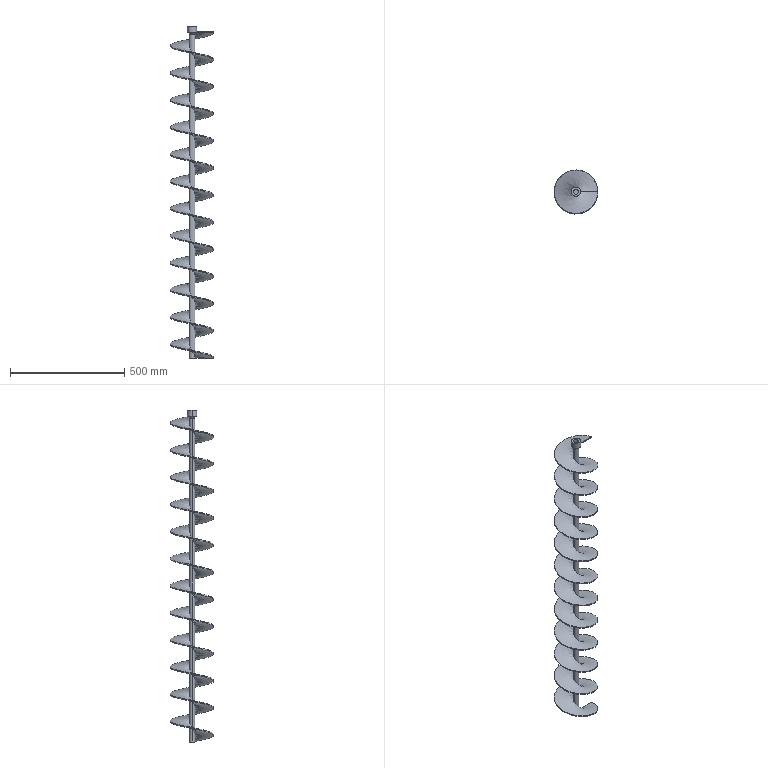Part | SolidWorks | features ICE 2, Chamfer 1, Extrusion 1, Helix 1, Sweep 1 | 1 solid | 42 faces | box 190 x 190 x 1450 mm | volume 2067937 mm3 | cylinder 30 | plane 6 | cone 3 | spline 3 | commonest cylinder face diameters 25 x26 22 x2 40 x2